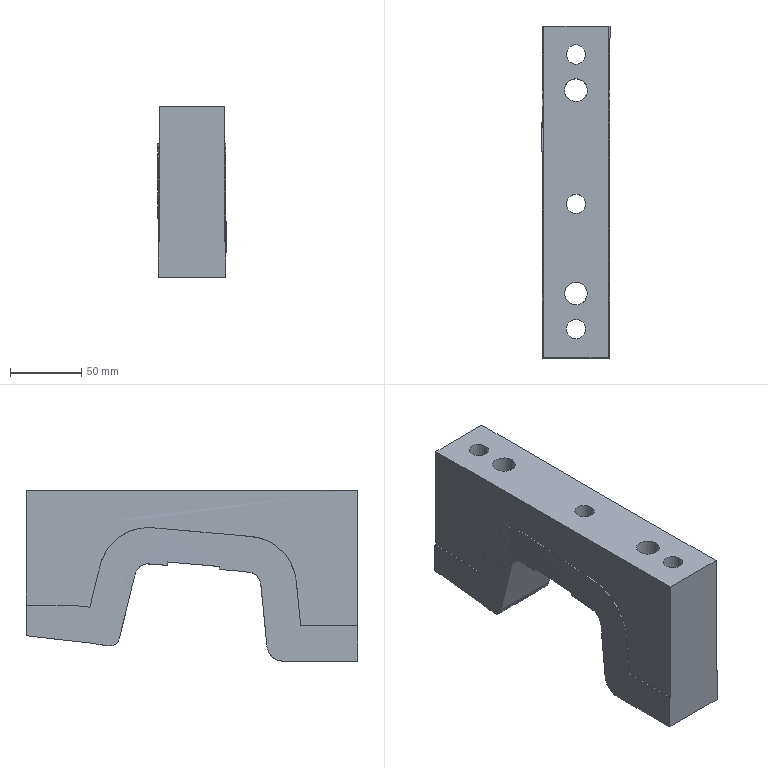Part | NX | features solid 2 | 1 solid | 42 faces | box 47.882 x 233 x 119.961 mm | volume 840014 mm3 | spline 20 | plane 14 | cylinder 8 | commonest cylinder face diameters 13.5 x3 19.5 x3 16 x2